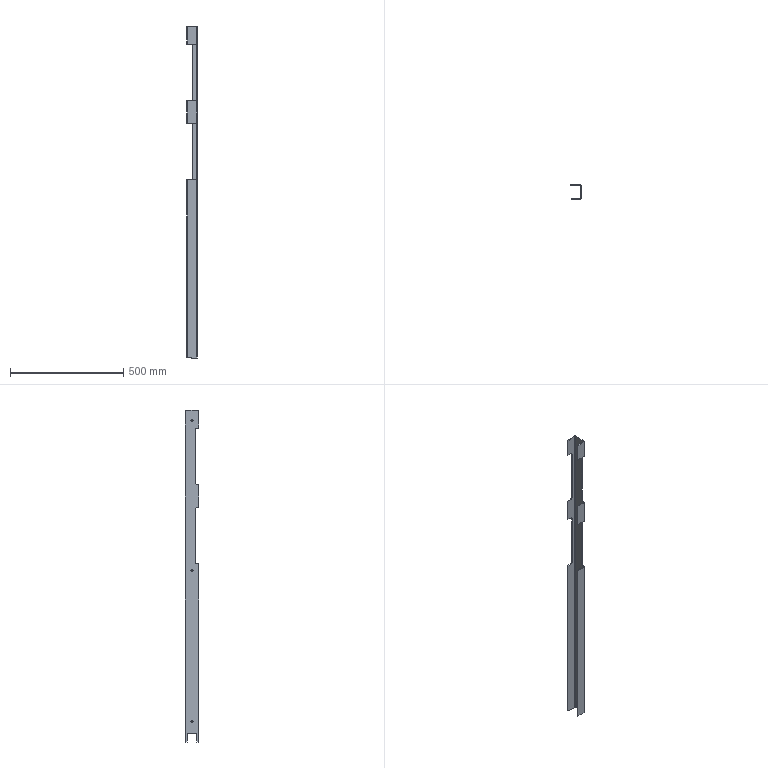Part | STEP file | Sliding Door Lower Rail Weldment | 1 solid | 324 faces | box 46 x 60 x 1467 mm | volume 339096 mm3 | plane 185 | spline 117 | cylinder 22 | commonest cylinder face diameters 20 x8 9 x6 0.2 x4 4.2 x4